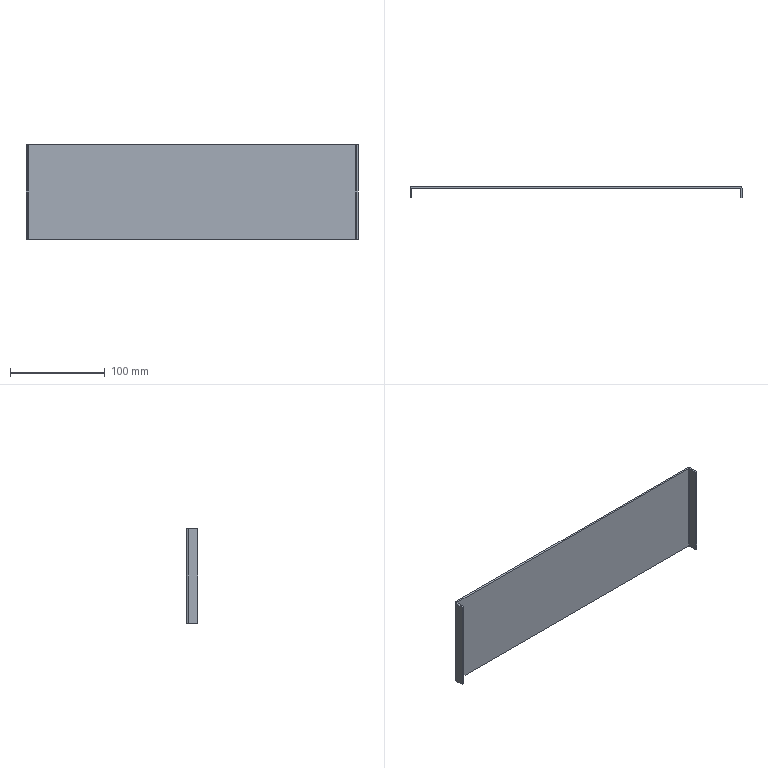Part | SolidWorks | features FlatPattern 1, SMBaseFlange 1, SheetMetal 1 | 1 solid | 22 faces | box 350 x 12 x 100 mm | volume 73794 mm3 | plane 18 | cylinder 4 | commonest cylinder face diameters 0.4 x2 4.4 x2
STEP:
#1=CARTESIAN_POINT('',(-172.8,0.,100.));
#2=VERTEX_POINT('',#1);
#3=CARTESIAN_POINT('',(-172.8,-2.,100.));
#4=VERTEX_POINT('',#3);
#5=CARTESIAN_POINT('',(-172.8,0.,100.));
#6=DIRECTION('',(0.,-1.,0.));
#7=VECTOR('',#6,1000.);
#8=LINE('',#5,#7);
#9=EDGE_CURVE('',#2,#4,#8,.T.);
#10=ORIENTED_EDGE('',*,*,#9,.F.);
#11=CARTESIAN_POINT('',(-175.,-2.2,100.));
#12=VERTEX_POINT('',#11);
#13=CARTESIAN_POINT('',(-172.8,-2.2,100.));
#14=DIRECTION('',(0.,0.,-1.));
#15=DIRECTION('',(1.,0.,0.));
#16=AXIS2_PLACEMENT_3D('',#13,#14,#15);
#17=CIRCLE('',#16,2.2);
#18=EDGE_CURVE('',#12,#2,#17,.T.);
#19=ORIENTED_EDGE('',*,*,#18,.F.);
#20=CARTESIAN_POINT('',(-173.,-2.2,100.));
#21=VERTEX_POINT('',#20);
#22=CARTESIAN_POINT('',(-173.,-2.2,100.));
#23=DIRECTION('',(-1.,0.,0.));
#24=VECTOR('',#23,1000.);
#25=LINE('',#22,#24);
#26=EDGE_CURVE('',#21,#12,#25,.T.);
#27=ORIENTED_EDGE('',*,*,#26,.F.);
#28=CARTESIAN_POINT('',(-172.8,-2.2,100.));
#29=DIRECTION('',(0.,0.,-1.));
#30=DIRECTION('',(1.,0.,0.));
#31=AXIS2_PLACEMENT_3D('',#28,#29,#30);
#32=CIRCLE('',#31,0.2);
#33=EDGE_CURVE('',#21,#4,#32,.T.);
#34=ORIENTED_EDGE('',*,*,#33,.T.);
#35=EDGE_LOOP('',(#10,#19,#27,#34));
#36=FACE_OUTER_BOUND('',#35,.T.);
#37=CARTESIAN_POINT('',(-172.8,0.,100.));
#38=DIRECTION('',(0.,0.,1.));
#39=DIRECTION('',(1.,0.,0.));
#40=AXIS2_PLACEMENT_3D('',#37,#38,#39);
#41=PLANE('',#40);
#42=ADVANCED_FACE('',(#36),#41,.T.);
#43=CARTESIAN_POINT('',(172.8,0.,100.));
#44=VERTEX_POINT('',#43);
#45=CARTESIAN_POINT('',(-175.,0.,100.));
#46=DIRECTION('',(1.,0.,0.));
#47=VECTOR('',#46,1000.);
#48=LINE('',#45,#47);
#49=EDGE_CURVE('',#2,#44,#48,.T.);
#50=ORIENTED_EDGE('',*,*,#49,.F.);
#51=ORIENTED_EDGE('',*,*,#9,.T.);
#52=CARTESIAN_POINT('',(172.8,-2.,100.));
#53=VERTEX_POINT('',#52);
#54=CARTESIAN_POINT('',(-175.,-2.,100.));
#55=DIRECTION('',(1.,0.,0.));
#56=VECTOR('',#55,1000.);
#57=LINE('',#54,#56);
#58=EDGE_CURVE('',#4,#53,#57,.T.);
#59=ORIENTED_EDGE('',*,*,#58,.T.);
#60=CARTESIAN_POINT('',(172.8,-2.,100.));
#61=DIRECTION('',(0.,1.,0.));
#62=VECTOR('',#61,1000.);
#63=LINE('',#60,#62);
#64=EDGE_CURVE('',#53,#44,#63,.T.);
#65=ORIENTED_EDGE('',*,*,#64,.T.);
#66=EDGE_LOOP('',(#50,#51,#59,#65));
#67=FACE_OUTER_BOUND('',#66,.T.);
#68=CARTESIAN_POINT('',(-173.,-2.2,100.));
#69=DIRECTION('',(0.,0.,1.));
#70=DIRECTION('',(1.,0.,0.));
#71=AXIS2_PLACEMENT_3D('',#68,#69,#70);
#72=PLANE('',#71);
#73=ADVANCED_FACE('',(#67),#72,.T.);
#74=CARTESIAN_POINT('',(-175.,-2.2,0.));
#75=VERTEX_POINT('',#74);
#76=CARTESIAN_POINT('',(-173.,-2.2,0.));
#77=VERTEX_POINT('',#76);
#78=CARTESIAN_POINT('',(-175.,-2.2,0.));
#79=DIRECTION('',(1.,0.,0.));
#80=VECTOR('',#79,1000.);
#81=LINE('',#78,#80);
#82=EDGE_CURVE('',#75,#77,#81,.T.);
#83=ORIENTED_EDGE('',*,*,#82,.F.);
#84=CARTESIAN_POINT('',(-172.8,0.,0.));
#85=VERTEX_POINT('',#84);
#86=CARTESIAN_POINT('',(-172.8,-2.2,0.));
#87=DIRECTION('',(0.,0.,-1.));
#88=DIRECTION('',(1.,0.,0.));
#89=AXIS2_PLACEMENT_3D('',#86,#87,#88);
#90=CIRCLE('',#89,2.2);
#91=EDGE_CURVE('',#75,#85,#90,.T.);
#92=ORIENTED_EDGE('',*,*,#91,.T.);
#93=CARTESIAN_POINT('',(-172.8,-2.,0.));
#94=VERTEX_POINT('',#93);
#95=CARTESIAN_POINT('',(-172.8,-2.,0.));
#96=DIRECTION('',(0.,1.,0.));
#97=VECTOR('',#96,1000.);
#98=LINE('',#95,#97);
#99=EDGE_CURVE('',#94,#85,#98,.T.);
#100=ORIENTED_EDGE('',*,*,#99,.F.);
#101=CARTESIAN_POINT('',(-172.8,-2.2,0.));
#102=DIRECTION('',(0.,0.,-1.));
#103=DIRECTION('',(1.,0.,0.));
#104=AXIS2_PLACEMENT_3D('',#101,#102,#103);
#105=CIRCLE('',#104,0.2);
#106=EDGE_CURVE('',#77,#94,#105,.T.);
#107=ORIENTED_EDGE('',*,*,#106,.F.);
#108=EDGE_LOOP('',(#83,#92,#100,#107));
#109=FACE_OUTER_BOUND('',#108,.T.);
#110=CARTESIAN_POINT('',(-175.,-2.2,0.));
#111=DIRECTION('',(0.,0.,-1.));
#112=DIRECTION('',(-1.,0.,0.));
#113=AXIS2_PLACEMENT_3D('',#110,#111,#112);
#114=PLANE('',#113);
#115=ADVANCED_FACE('',(#109),#114,.T.);
#116=CARTESIAN_POINT('',(-175.,-12.,0.));
#117=VERTEX_POINT('',#116);
#118=CARTESIAN_POINT('',(-175.,-12.,0.));
#119=DIRECTION('',(0.,1.,0.));
#120=VECTOR('',#119,1000.);
#121=LINE('',#118,#120);
#122=EDGE_CURVE('',#117,#75,#121,.T.);
#123=ORIENTED_EDGE('',*,*,#122,.T.);
#124=ORIENTED_EDGE('',*,*,#82,.T.);
#125=CARTESIAN_POINT('',(-173.,-12.,0.));
#126=VERTEX_POINT('',#125);
#127=CARTESIAN_POINT('',(-173.,-12.,0.));
#128=DIRECTION('',(0.,1.,0.));
#129=VECTOR('',#128,1000.);
#130=LINE('',#127,#129);
#131=EDGE_CURVE('',#126,#77,#130,.T.);
#132=ORIENTED_EDGE('',*,*,#131,.F.);
#133=CARTESIAN_POINT('',(-173.,-12.,0.));
#134=DIRECTION('',(-1.,0.,0.));
#135=VECTOR('',#134,1000.);
#136=LINE('',#133,#135);
#137=EDGE_CURVE('',#126,#117,#136,.T.);
#138=ORIENTED_EDGE('',*,*,#137,.T.);
#139=EDGE_LOOP('',(#123,#124,#132,#138));
#140=FACE_OUTER_BOUND('',#139,.T.);
#141=CARTESIAN_POINT('',(-172.8,-2.,0.));
#142=DIRECTION('',(0.,0.,-1.));
#143=DIRECTION('',(-1.,0.,0.));
#144=AXIS2_PLACEMENT_3D('',#141,#142,#143);
#145=PLANE('',#144);
#146=ADVANCED_FACE('',(#140),#145,.T.);
#147=CARTESIAN_POINT('',(175.,-2.2,100.));
#148=VERTEX_POINT('',#147);
#149=CARTESIAN_POINT('',(173.,-2.2,100.));
#150=VERTEX_POINT('',#149);
#151=CARTESIAN_POINT('',(175.,-2.2,100.));
#152=DIRECTION('',(-1.,0.,0.));
#153=VECTOR('',#152,1000.);
#154=LINE('',#151,#153);
#155=EDGE_CURVE('',#148,#150,#154,.T.);
#156=ORIENTED_EDGE('',*,*,#155,.F.);
#157=CARTESIAN_POINT('',(172.8,-2.2,100.));
#158=DIRECTION('',(0.,0.,-1.));
#159=DIRECTION('',(1.,0.,0.));
#160=AXIS2_PLACEMENT_3D('',#157,#158,#159);
#161=CIRCLE('',#160,2.2);
#162=EDGE_CURVE('',#44,#148,#161,.T.);
#163=ORIENTED_EDGE('',*,*,#162,.F.);
#164=ORIENTED_EDGE('',*,*,#64,.F.);
#165=CARTESIAN_POINT('',(172.8,-2.2,100.));
#166=DIRECTION('',(0.,0.,-1.));
#167=DIRECTION('',(1.,0.,0.));
#168=AXIS2_PLACEMENT_3D('',#165,#166,#167);
#169=CIRCLE('',#168,0.2);
#170=EDGE_CURVE('',#53,#150,#169,.T.);
#171=ORIENTED_EDGE('',*,*,#170,.T.);
#172=EDGE_LOOP('',(#156,#163,#164,#171));
#173=FACE_OUTER_BOUND('',#172,.T.);
#174=CARTESIAN_POINT('',(175.,-2.2,100.));
#175=DIRECTION('',(0.,0.,1.));
#176=DIRECTION('',(1.,0.,0.));
#177=AXIS2_PLACEMENT_3D('',#174,#175,#176);
#178=PLANE('',#177);
#179=ADVANCED_FACE('',(#173),#178,.T.);
#180=CARTESIAN_POINT('',(175.,-12.,100.));
#181=VERTEX_POINT('',#180);
#182=CARTESIAN_POINT('',(175.,0.,100.));
#183=DIRECTION('',(0.,-1.,0.));
#184=VECTOR('',#183,1000.);
#185=LINE('',#182,#184);
#186=EDGE_CURVE('',#148,#181,#185,.T.);
#187=ORIENTED_EDGE('',*,*,#186,.F.);
#188=ORIENTED_EDGE('',*,*,#155,.T.);
#189=CARTESIAN_POINT('',(173.,-12.,100.));
#190=VERTEX_POINT('',#189);
#191=CARTESIAN_POINT('',(173.,0.,100.));
#192=DIRECTION('',(0.,-1.,0.));
#193=VECTOR('',#192,1000.);
#194=LINE('',#191,#193);
#195=EDGE_CURVE('',#150,#190,#194,.T.);
#196=ORIENTED_EDGE('',*,*,#195,.T.);
#197=CARTESIAN_POINT('',(175.,-12.,100.));
#198=DIRECTION('',(-1.,0.,0.));
#199=VECTOR('',#198,1000.);
#200=LINE('',#197,#199);
#201=EDGE_CURVE('',#181,#190,#200,.T.);
#202=ORIENTED_EDGE('',*,*,#201,.F.);
#203=EDGE_LOOP('',(#187,#188,#196,#202));
#204=FACE_OUTER_BOUND('',#203,.T.);
#205=CARTESIAN_POINT('',(172.8,-2.,100.));
#206=DIRECTION('',(0.,0.,1.));
#207=DIRECTION('',(1.,0.,0.));
#208=AXIS2_PLACEMENT_3D('',#205,#206,#207);
#209=PLANE('',#208);
#210=ADVANCED_FACE('',(#204),#209,.T.);
#211=CARTESIAN_POINT('',(172.8,0.,0.));
#212=VERTEX_POINT('',#211);
#213=CARTESIAN_POINT('',(172.8,-2.,0.));
#214=VERTEX_POINT('',#213);
#215=CARTESIAN_POINT('',(172.8,0.,0.));
#216=DIRECTION('',(0.,-1.,0.));
#217=VECTOR('',#216,1000.);
#218=LINE('',#215,#217);
#219=EDGE_CURVE('',#212,#214,#218,.T.);
#220=ORIENTED_EDGE('',*,*,#219,.F.);
#221=CARTESIAN_POINT('',(175.,-2.2,0.));
#222=VERTEX_POINT('',#221);
#223=CARTESIAN_POINT('',(172.8,-2.2,0.));
#224=DIRECTION('',(0.,0.,-1.));
#225=DIRECTION('',(1.,0.,0.));
#226=AXIS2_PLACEMENT_3D('',#223,#224,#225);
#227=CIRCLE('',#226,2.2);
#228=EDGE_CURVE('',#212,#222,#227,.T.);
#229=ORIENTED_EDGE('',*,*,#228,.T.);
#230=CARTESIAN_POINT('',(173.,-2.2,0.));
#231=VERTEX_POINT('',#230);
#232=CARTESIAN_POINT('',(173.,-2.2,0.));
#233=DIRECTION('',(1.,0.,0.));
#234=VECTOR('',#233,1000.);
#235=LINE('',#232,#234);
#236=EDGE_CURVE('',#231,#222,#235,.T.);
#237=ORIENTED_EDGE('',*,*,#236,.F.);
#238=CARTESIAN_POINT('',(172.8,-2.2,0.));
#239=DIRECTION('',(0.,0.,-1.));
#240=DIRECTION('',(1.,0.,0.));
#241=AXIS2_PLACEMENT_3D('',#238,#239,#240);
#242=CIRCLE('',#241,0.2);
#243=EDGE_CURVE('',#214,#231,#242,.T.);
#244=ORIENTED_EDGE('',*,*,#243,.F.);
#245=EDGE_LOOP('',(#220,#229,#237,#244));
#246=FACE_OUTER_BOUND('',#245,.T.);
#247=CARTESIAN_POINT('',(172.8,0.,0.));
#248=DIRECTION('',(0.,0.,-1.));
#249=DIRECTION('',(-1.,0.,0.));
#250=AXIS2_PLACEMENT_3D('',#247,#248,#249);
#251=PLANE('',#250);
#252=ADVANCED_FACE('',(#246),#251,.T.);
#253=CARTESIAN_POINT('',(-175.,0.,0.));
#254=DIRECTION('',(1.,0.,0.));
#255=VECTOR('',#254,1000.);
#256=LINE('',#253,#255);
#257=EDGE_CURVE('',#85,#212,#256,.T.);
#258=ORIENTED_EDGE('',*,*,#257,.T.);
#259=ORIENTED_EDGE('',*,*,#219,.T.);
#260=CARTESIAN_POINT('',(-175.,-2.,0.));
#261=DIRECTION('',(1.,0.,0.));
#262=VECTOR('',#261,1000.);
#263=LINE('',#260,#262);
#264=EDGE_CURVE('',#94,#214,#263,.T.);
#265=ORIENTED_EDGE('',*,*,#264,.F.);
#266=ORIENTED_EDGE('',*,*,#99,.T.);
#267=EDGE_LOOP('',(#258,#259,#265,#266));
#268=FACE_OUTER_BOUND('',#267,.T.);
#269=CARTESIAN_POINT('',(173.,-2.2,0.));
#270=DIRECTION('',(0.,0.,-1.));
#271=DIRECTION('',(-1.,0.,0.));
#272=AXIS2_PLACEMENT_3D('',#269,#270,#271);
#273=PLANE('',#272);
#274=ADVANCED_FACE('',(#268),#273,.T.);
#275=CARTESIAN_POINT('',(173.,-12.,0.));
#276=VERTEX_POINT('',#275);
#277=CARTESIAN_POINT('',(173.,0.,0.));
#278=DIRECTION('',(0.,-1.,0.));
#279=VECTOR('',#278,1000.);
#280=LINE('',#277,#279);
#281=EDGE_CURVE('',#231,#276,#280,.T.);
#282=ORIENTED_EDGE('',*,*,#281,.T.);
#283=CARTESIAN_POINT('',(173.,-12.,100.));
#284=DIRECTION('',(0.,0.,-1.));
#285=VECTOR('',#284,1000.);
#286=LINE('',#283,#285);
#287=EDGE_CURVE('',#190,#276,#286,.T.);
#288=ORIENTED_EDGE('',*,*,#287,.F.);
#289=ORIENTED_EDGE('',*,*,#195,.F.);
#290=CARTESIAN_POINT('',(173.,-2.2,100.));
#291=DIRECTION('',(0.,0.,-1.));
#292=VECTOR('',#291,1000.);
#293=LINE('',#290,#292);
#294=EDGE_CURVE('',#150,#231,#293,.T.);
#295=ORIENTED_EDGE('',*,*,#294,.T.);
#296=EDGE_LOOP('',(#282,#288,#289,#295));
#297=FACE_OUTER_BOUND('',#296,.T.);
#298=CARTESIAN_POINT('',(173.,0.,100.));
#299=DIRECTION('',(1.,0.,0.));
#300=DIRECTION('',(0.,0.,-1.));
#301=AXIS2_PLACEMENT_3D('',#298,#299,#300);
#302=PLANE('',#301);
#303=ADVANCED_FACE('',(#297),#302,.F.);
#304=CARTESIAN_POINT('',(175.,-12.,0.));
#305=VERTEX_POINT('',#304);
#306=CARTESIAN_POINT('',(175.,-12.,0.));
#307=DIRECTION('',(-1.,0.,0.));
#308=VECTOR('',#307,1000.);
#309=LINE('',#306,#308);
#310=EDGE_CURVE('',#305,#276,#309,.T.);
#311=ORIENTED_EDGE('',*,*,#310,.F.);
#312=CARTESIAN_POINT('',(175.,-12.,100.));
#313=DIRECTION('',(0.,0.,-1.));
#314=VECTOR('',#313,1000.);
#315=LINE('',#312,#314);
#316=EDGE_CURVE('',#181,#305,#315,.T.);
#317=ORIENTED_EDGE('',*,*,#316,.F.);
#318=ORIENTED_EDGE('',*,*,#201,.T.);
#319=ORIENTED_EDGE('',*,*,#287,.T.);
#320=EDGE_LOOP('',(#311,#317,#318,#319));
#321=FACE_OUTER_BOUND('',#320,.T.);
#322=CARTESIAN_POINT('',(175.,-12.,100.));
#323=DIRECTION('',(0.,-1.,0.));
#324=DIRECTION('',(0.,0.,-1.));
#325=AXIS2_PLACEMENT_3D('',#322,#323,#324);
#326=PLANE('',#325);
#327=ADVANCED_FACE('',(#321),#326,.T.);
#328=CARTESIAN_POINT('',(175.,0.,0.));
#329=DIRECTION('',(0.,-1.,0.));
#330=VECTOR('',#329,1000.);
#331=LINE('',#328,#330);
#332=EDGE_CURVE('',#222,#305,#331,.T.);
#333=ORIENTED_EDGE('',*,*,#332,.F.);
#334=CARTESIAN_POINT('',(175.,-2.2,100.));
#335=DIRECTION('',(0.,0.,-1.));
#336=VECTOR('',#335,1000.);
#337=LINE('',#334,#336);
#338=EDGE_CURVE('',#148,#222,#337,.T.);
#339=ORIENTED_EDGE('',*,*,#338,.F.);
#340=ORIENTED_EDGE('',*,*,#186,.T.);
#341=ORIENTED_EDGE('',*,*,#316,.T.);
#342=EDGE_LOOP('',(#333,#339,#340,#341));
#343=FACE_OUTER_BOUND('',#342,.T.);
#344=CARTESIAN_POINT('',(175.,0.,100.));
#345=DIRECTION('',(1.,0.,0.));
#346=DIRECTION('',(0.,0.,-1.));
#347=AXIS2_PLACEMENT_3D('',#344,#345,#346);
#348=PLANE('',#347);
#349=ADVANCED_FACE('',(#343),#348,.T.);
#350=ORIENTED_EDGE('',*,*,#228,.F.);
#351=CARTESIAN_POINT('',(172.8,0.,100.));
#352=DIRECTION('',(0.,0.,-1.));
#353=VECTOR('',#352,1000.);
#354=LINE('',#351,#353);
#355=EDGE_CURVE('',#44,#212,#354,.T.);
#356=ORIENTED_EDGE('',*,*,#355,.F.);
#357=ORIENTED_EDGE('',*,*,#162,.T.);
#358=ORIENTED_EDGE('',*,*,#338,.T.);
#359=EDGE_LOOP('',(#350,#356,#357,#358));
#360=FACE_OUTER_BOUND('',#359,.T.);
#361=CARTESIAN_POINT('',(172.8,-2.2,100.));
#362=DIRECTION('',(0.,0.,-1.));
#363=DIRECTION('',(-1.,0.,0.));
#364=AXIS2_PLACEMENT_3D('',#361,#362,#363);
#365=CYLINDRICAL_SURFACE('',#364,2.2);
#366=ADVANCED_FACE('',(#360),#365,.T.);
#367=ORIENTED_EDGE('',*,*,#257,.F.);
#368=CARTESIAN_POINT('',(-172.8,0.,100.));
#369=DIRECTION('',(0.,0.,-1.));
#370=VECTOR('',#369,1000.);
#371=LINE('',#368,#370);
#372=EDGE_CURVE('',#2,#85,#371,.T.);
#373=ORIENTED_EDGE('',*,*,#372,.F.);
#374=ORIENTED_EDGE('',*,*,#49,.T.);
#375=ORIENTED_EDGE('',*,*,#355,.T.);
#376=EDGE_LOOP('',(#367,#373,#374,#375));
#377=FACE_OUTER_BOUND('',#376,.T.);
#378=CARTESIAN_POINT('',(-175.,0.,100.));
#379=DIRECTION('',(0.,1.,0.));
#380=DIRECTION('',(0.,0.,1.));
#381=AXIS2_PLACEMENT_3D('',#378,#379,#380);
#382=PLANE('',#381);
#383=ADVANCED_FACE('',(#377),#382,.T.);
#384=ORIENTED_EDGE('',*,*,#91,.F.);
#385=CARTESIAN_POINT('',(-175.,-2.2,100.));
#386=DIRECTION('',(0.,0.,-1.));
#387=VECTOR('',#386,1000.);
#388=LINE('',#385,#387);
#389=EDGE_CURVE('',#12,#75,#388,.T.);
#390=ORIENTED_EDGE('',*,*,#389,.F.);
#391=ORIENTED_EDGE('',*,*,#18,.T.);
#392=ORIENTED_EDGE('',*,*,#372,.T.);
#393=EDGE_LOOP('',(#384,#390,#391,#392));
#394=FACE_OUTER_BOUND('',#393,.T.);
#395=CARTESIAN_POINT('',(-172.8,-2.2,100.));
#396=DIRECTION('',(0.,0.,-1.));
#397=DIRECTION('',(-1.,0.,0.));
#398=AXIS2_PLACEMENT_3D('',#395,#396,#397);
#399=CYLINDRICAL_SURFACE('',#398,2.2);
#400=ADVANCED_FACE('',(#394),#399,.T.);
#401=ORIENTED_EDGE('',*,*,#122,.F.);
#402=CARTESIAN_POINT('',(-175.,-12.,100.));
#403=VERTEX_POINT('',#402);
#404=CARTESIAN_POINT('',(-175.,-12.,100.));
#405=DIRECTION('',(0.,0.,-1.));
#406=VECTOR('',#405,1000.);
#407=LINE('',#404,#406);
#408=EDGE_CURVE('',#403,#117,#407,.T.);
#409=ORIENTED_EDGE('',*,*,#408,.F.);
#410=CARTESIAN_POINT('',(-175.,-12.,100.));
#411=DIRECTION('',(0.,1.,0.));
#412=VECTOR('',#411,1000.);
#413=LINE('',#410,#412);
#414=EDGE_CURVE('',#403,#12,#413,.T.);
#415=ORIENTED_EDGE('',*,*,#414,.T.);
#416=ORIENTED_EDGE('',*,*,#389,.T.);
#417=EDGE_LOOP('',(#401,#409,#415,#416));
#418=FACE_OUTER_BOUND('',#417,.T.);
#419=CARTESIAN_POINT('',(-175.,-12.,100.));
#420=DIRECTION('',(-1.,0.,0.));
#421=DIRECTION('',(0.,0.,1.));
#422=AXIS2_PLACEMENT_3D('',#419,#420,#421);
#423=PLANE('',#422);
#424=ADVANCED_FACE('',(#418),#423,.T.);
#425=ORIENTED_EDGE('',*,*,#137,.F.);
#426=CARTESIAN_POINT('',(-173.,-12.,100.));
#427=VERTEX_POINT('',#426);
#428=CARTESIAN_POINT('',(-173.,-12.,100.));
#429=DIRECTION('',(0.,0.,-1.));
#430=VECTOR('',#429,1000.);
#431=LINE('',#428,#430);
#432=EDGE_CURVE('',#427,#126,#431,.T.);
#433=ORIENTED_EDGE('',*,*,#432,.F.);
#434=CARTESIAN_POINT('',(-173.,-12.,100.));
#435=DIRECTION('',(-1.,0.,0.));
#436=VECTOR('',#435,1000.);
#437=LINE('',#434,#436);
#438=EDGE_CURVE('',#427,#403,#437,.T.);
#439=ORIENTED_EDGE('',*,*,#438,.T.);
#440=ORIENTED_EDGE('',*,*,#408,.T.);
#441=EDGE_LOOP('',(#425,#433,#439,#440));
#442=FACE_OUTER_BOUND('',#441,.T.);
#443=CARTESIAN_POINT('',(-173.,-12.,100.));
#444=DIRECTION('',(0.,-1.,0.));
#445=DIRECTION('',(0.,0.,-1.));
#446=AXIS2_PLACEMENT_3D('',#443,#444,#445);
#447=PLANE('',#446);
#448=ADVANCED_FACE('',(#442),#447,.T.);
#449=ORIENTED_EDGE('',*,*,#131,.T.);
#450=CARTESIAN_POINT('',(-173.,-2.2,100.));
#451=DIRECTION('',(0.,0.,-1.));
#452=VECTOR('',#451,1000.);
#453=LINE('',#450,#452);
#454=EDGE_CURVE('',#21,#77,#453,.T.);
#455=ORIENTED_EDGE('',*,*,#454,.F.);
#456=CARTESIAN_POINT('',(-173.,-12.,100.));
#457=DIRECTION('',(0.,1.,0.));
#458=VECTOR('',#457,1000.);
#459=LINE('',#456,#458);
#460=EDGE_CURVE('',#427,#21,#459,.T.);
#461=ORIENTED_EDGE('',*,*,#460,.F.);
#462=ORIENTED_EDGE('',*,*,#432,.T.);
#463=EDGE_LOOP('',(#449,#455,#461,#462));
#464=FACE_OUTER_BOUND('',#463,.T.);
#465=CARTESIAN_POINT('',(-173.,-12.,100.));
#466=DIRECTION('',(-1.,0.,0.));
#467=DIRECTION('',(0.,0.,1.));
#468=AXIS2_PLACEMENT_3D('',#465,#466,#467);
#469=PLANE('',#468);
#470=ADVANCED_FACE('',(#464),#469,.F.);
#471=ORIENTED_EDGE('',*,*,#106,.T.);
#472=CARTESIAN_POINT('',(-172.8,-2.,100.));
#473=DIRECTION('',(0.,0.,-1.));
#474=VECTOR('',#473,1000.);
#475=LINE('',#472,#474);
#476=EDGE_CURVE('',#4,#94,#475,.T.);
#477=ORIENTED_EDGE('',*,*,#476,.F.);
#478=ORIENTED_EDGE('',*,*,#33,.F.);
#479=ORIENTED_EDGE('',*,*,#454,.T.);
#480=EDGE_LOOP('',(#471,#477,#478,#479));
#481=FACE_OUTER_BOUND('',#480,.T.);
#482=CARTESIAN_POINT('',(-172.8,-2.2,100.));
#483=DIRECTION('',(0.,0.,-1.));
#484=DIRECTION('',(-1.,0.,0.));
#485=AXIS2_PLACEMENT_3D('',#482,#483,#484);
#486=CYLINDRICAL_SURFACE('',#485,0.2);
#487=ADVANCED_FACE('',(#481),#486,.F.);
#488=ORIENTED_EDGE('',*,*,#264,.T.);
#489=CARTESIAN_POINT('',(172.8,-2.,100.));
#490=DIRECTION('',(0.,0.,-1.));
#491=VECTOR('',#490,1000.);
#492=LINE('',#489,#491);
#493=EDGE_CURVE('',#53,#214,#492,.T.);
#494=ORIENTED_EDGE('',*,*,#493,.F.);
#495=ORIENTED_EDGE('',*,*,#58,.F.);
#496=ORIENTED_EDGE('',*,*,#476,.T.);
#497=EDGE_LOOP('',(#488,#494,#495,#496));
#498=FACE_OUTER_BOUND('',#497,.T.);
#499=CARTESIAN_POINT('',(-175.,-2.,100.));
#500=DIRECTION('',(0.,1.,0.));
#501=DIRECTION('',(0.,0.,1.));
#502=AXIS2_PLACEMENT_3D('',#499,#500,#501);
#503=PLANE('',#502);
#504=ADVANCED_FACE('',(#498),#503,.F.);
#505=ORIENTED_EDGE('',*,*,#243,.T.);
#506=ORIENTED_EDGE('',*,*,#294,.F.);
#507=ORIENTED_EDGE('',*,*,#170,.F.);
#508=ORIENTED_EDGE('',*,*,#493,.T.);
#509=EDGE_LOOP('',(#505,#506,#507,#508));
#510=FACE_OUTER_BOUND('',#509,.T.);
#511=CARTESIAN_POINT('',(172.8,-2.2,100.));
#512=DIRECTION('',(0.,0.,-1.));
#513=DIRECTION('',(-1.,0.,0.));
#514=AXIS2_PLACEMENT_3D('',#511,#512,#513);
#515=CYLINDRICAL_SURFACE('',#514,0.2);
#516=ADVANCED_FACE('',(#510),#515,.F.);
#517=ORIENTED_EDGE('',*,*,#460,.T.);
#518=ORIENTED_EDGE('',*,*,#26,.T.);
#519=ORIENTED_EDGE('',*,*,#414,.F.);
#520=ORIENTED_EDGE('',*,*,#438,.F.);
#521=EDGE_LOOP('',(#517,#518,#519,#520));
#522=FACE_OUTER_BOUND('',#521,.T.);
#523=CARTESIAN_POINT('',(172.8,-2.2,100.));
#524=DIRECTION('',(0.,0.,1.));
#525=DIRECTION('',(1.,0.,0.));
#526=AXIS2_PLACEMENT_3D('',#523,#524,#525);
#527=PLANE('',#526);
#528=ADVANCED_FACE('',(#522),#527,.T.);
#529=ORIENTED_EDGE('',*,*,#281,.F.);
#530=ORIENTED_EDGE('',*,*,#236,.T.);
#531=ORIENTED_EDGE('',*,*,#332,.T.);
#532=ORIENTED_EDGE('',*,*,#310,.T.);
#533=EDGE_LOOP('',(#529,#530,#531,#532));
#534=FACE_OUTER_BOUND('',#533,.T.);
#535=CARTESIAN_POINT('',(172.8,-2.2,0.));
#536=DIRECTION('',(0.,0.,1.));
#537=DIRECTION('',(1.,0.,0.));
#538=AXIS2_PLACEMENT_3D('',#535,#536,#537);
#539=PLANE('',#538);
#540=ADVANCED_FACE('',(#534),#539,.F.);
#541=CLOSED_SHELL('',(#42,#73,#115,#146,#179,#210,#252,#274,#303,#327,#349,#366,#383,#400,#424,#448,#470,#487,#504,#516,#528,#540));
#542=MANIFOLD_SOLID_BREP('',#541);
#543=CARTESIAN_POINT('',(0.,0.,0.));
#544=DIRECTION('',(0.,0.,1.));
#545=DIRECTION('',(1.,0.,0.));
#546=AXIS2_PLACEMENT_3D('',#543,#544,#545);
#547=(LENGTH_UNIT()NAMED_UNIT(*)SI_UNIT(.MILLI.,.METRE.));
#548=UNCERTAINTY_MEASURE_WITH_UNIT(LENGTH_MEASURE(0.00001),#547,'','');
#549=(NAMED_UNIT(*)PLANE_ANGLE_UNIT()SI_UNIT($,.RADIAN.));
#550=(NAMED_UNIT(*)SI_UNIT($,.STERADIAN.)SOLID_ANGLE_UNIT());
#551=(GEOMETRIC_REPRESENTATION_CONTEXT(3)GLOBAL_UNCERTAINTY_ASSIGNED_CONTEXT((#548))GLOBAL_UNIT_ASSIGNED_CONTEXT((#547,#549,#550))REPRESENTATION_CONTEXT('',''));
#552=ADVANCED_BREP_SHAPE_REPRESENTATION('',(#542,#546),#551);